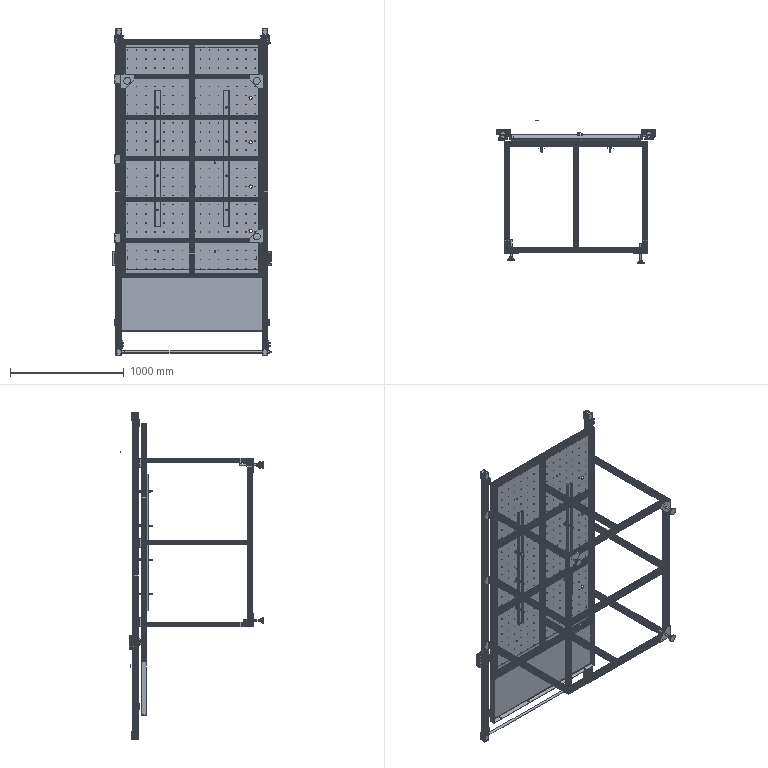Part | SolidWorks | features ReferencePattern 5, InContextFeatHolder 2, LocalLPattern 1, MirrorCompFeat 1 | 130 solids | 16854 faces | volume 36230878 mm3 | plane 8773 | cylinder 5258 | cone 2071 | spline 540 | torus 188 | sphere 24 | commonest cylinder face diameters 4 x899 0.2 x764 1 x570 2 x269 0.4 x238 5.5 x234